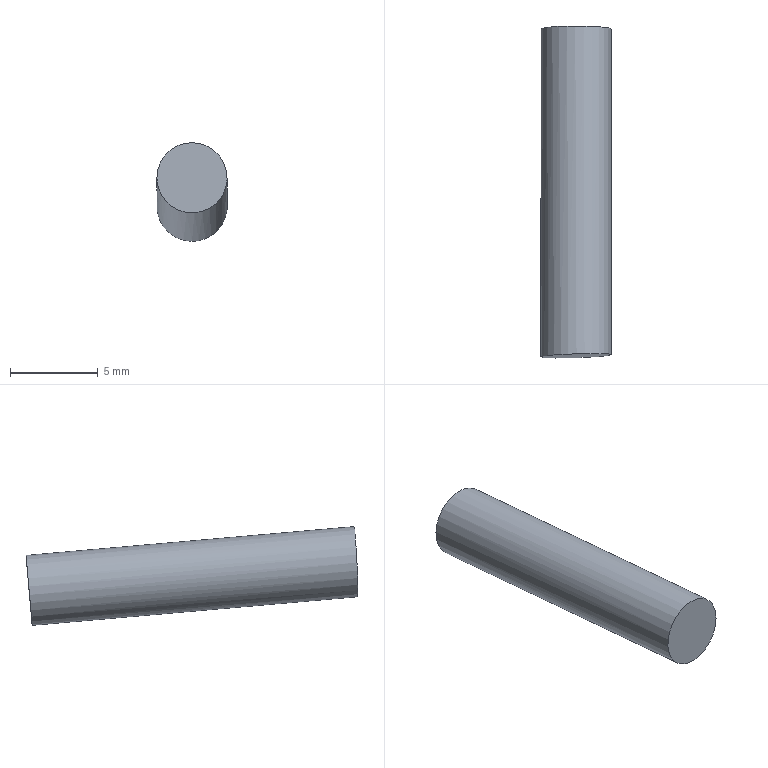Part | NX | features solid 2 | 1 solid | 3 faces | box 4 x 18.898 x 5.618 mm | volume 234.616 mm3 | plane 2 | cylinder 1 | commonest cylinder face diameters 4 x1
STEP:
#1=CARTESIAN_POINT('',(-561.105,-50.227,-39.442));
#2=VERTEX_POINT('',#1);
#3=CARTESIAN_POINT('',(-561.105,-50.053,-37.45));
#4=DIRECTION('',(0.,-0.9962,0.08716));
#5=DIRECTION('',(0.,-0.08716,-0.9962));
#6=AXIS2_PLACEMENT_3D('',#3,#4,#5);
#7=CIRCLE('',#6,2.);
#8=EDGE_CURVE('',#2,#2,#7,.T.);
#9=ORIENTED_EDGE('',*,*,#8,.F.);
#10=EDGE_LOOP('',(#9));
#11=FACE_BOUND('',#10,.T.);
#12=CARTESIAN_POINT('',(-561.105,-50.053,-37.45));
#13=DIRECTION('',(0.,0.9962,-0.08716));
#14=DIRECTION('',(0.,0.08716,0.9962));
#15=AXIS2_PLACEMENT_3D('',#12,#13,#14);
#16=PLANE('',#15);
#17=ADVANCED_FACE('',(#11),#16,.T.);
#18=CARTESIAN_POINT('',(-559.725,-68.684,-37.273));
#19=VERTEX_POINT('',#18);
#20=CARTESIAN_POINT('',(-561.105,-68.652,-35.823));
#21=DIRECTION('',(-0.03252,0.9981,-0.05307));
#22=DIRECTION('',(0.6892,-0.01607,-0.7244));
#23=AXIS2_PLACEMENT_3D('',#20,#21,#22);
#24=ELLIPSE('',#23,2.002,2.);
#25=EDGE_CURVE('',#19,#19,#24,.T.);
#26=ORIENTED_EDGE('',*,*,#25,.F.);
#27=EDGE_LOOP('',(#26));
#28=FACE_BOUND('',#27,.T.);
#29=CARTESIAN_POINT('',(-422.194,-57.948,80.353));
#30=DIRECTION('',(-0.03252,0.9981,-0.05307));
#31=DIRECTION('',(0.05223,-0.05133,-0.9973));
#32=AXIS2_PLACEMENT_3D('',#29,#30,#31);
#33=PLANE('',#32);
#34=ADVANCED_FACE('',(#28),#33,.F.);
#35=ORIENTED_EDGE('',*,*,#8,.T.);
#36=EDGE_LOOP('',(#35));
#37=FACE_BOUND('',#36,.T.);
#38=ORIENTED_EDGE('',*,*,#25,.T.);
#39=EDGE_LOOP('',(#38));
#40=FACE_BOUND('',#39,.T.);
#41=CARTESIAN_POINT('',(-561.105,-69.977,-35.707));
#42=DIRECTION('',(0.,0.9962,-0.08716));
#43=DIRECTION('',(0.,0.08716,0.9962));
#44=AXIS2_PLACEMENT_3D('',#41,#42,#43);
#45=CYLINDRICAL_SURFACE('',#44,2.);
#46=ADVANCED_FACE('',(#37,#40),#45,.T.);
#47=CLOSED_SHELL('',(#17,#34,#46));
#48=MANIFOLD_SOLID_BREP('',#47);
#49=(LENGTH_UNIT()NAMED_UNIT(*)SI_UNIT(.MILLI.,.METRE.));
#50=UNCERTAINTY_MEASURE_WITH_UNIT(LENGTH_MEASURE(0.00001),#49,'','');
#51=(NAMED_UNIT(*)PLANE_ANGLE_UNIT()SI_UNIT($,.RADIAN.));
#52=(NAMED_UNIT(*)SI_UNIT($,.STERADIAN.)SOLID_ANGLE_UNIT());
#53=(GEOMETRIC_REPRESENTATION_CONTEXT(3)GLOBAL_UNCERTAINTY_ASSIGNED_CONTEXT((#50))GLOBAL_UNIT_ASSIGNED_CONTEXT((#49,#51,#52))REPRESENTATION_CONTEXT('',''));
#54=ADVANCED_BREP_SHAPE_REPRESENTATION('',(#48),#53);